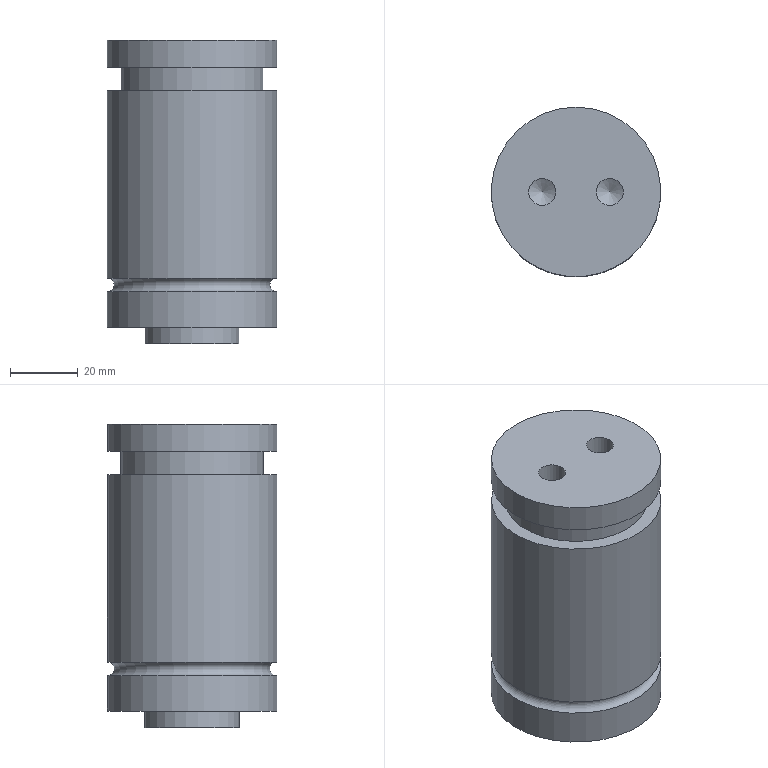Part | NX | features solid 2 | 1 solid | 15 faces | box 50.2 x 50.2 x 90 mm | volume 165612 mm3 | cylinder 7 | plane 5 | cone 2 | torus 1 | commonest cylinder face diameters 50.2 x3 8 x2 28 x1 42.2 x1
STEP:
#1=CARTESIAN_POINT('',(-615.,-166.,230.));
#2=VERTEX_POINT('',#1);
#3=CARTESIAN_POINT('',(-615.,-180.,230.));
#4=DIRECTION('',(0.,0.,1.));
#5=DIRECTION('',(0.,1.,0.));
#6=AXIS2_PLACEMENT_3D('',#3,#4,#5);
#7=CIRCLE('',#6,14.);
#8=EDGE_CURVE('',#2,#2,#7,.T.);
#9=ORIENTED_EDGE('',*,*,#8,.T.);
#10=EDGE_LOOP('',(#9));
#11=FACE_BOUND('',#10,.T.);
#12=CARTESIAN_POINT('',(-615.,-166.,235.));
#13=VERTEX_POINT('',#12);
#14=CARTESIAN_POINT('',(-615.,-180.,235.));
#15=DIRECTION('',(0.,0.,1.));
#16=DIRECTION('',(0.,1.,0.));
#17=AXIS2_PLACEMENT_3D('',#14,#15,#16);
#18=CIRCLE('',#17,14.);
#19=EDGE_CURVE('',#13,#13,#18,.T.);
#20=ORIENTED_EDGE('',*,*,#19,.F.);
#21=EDGE_LOOP('',(#20));
#22=FACE_BOUND('',#21,.T.);
#23=CARTESIAN_POINT('',(-615.,-180.,320.));
#24=DIRECTION('',(0.,0.,-1.));
#25=DIRECTION('',(0.,1.,0.));
#26=AXIS2_PLACEMENT_3D('',#23,#24,#25);
#27=CYLINDRICAL_SURFACE('',#26,14.);
#28=ADVANCED_FACE('',(#11,#22),#27,.T.);
#29=CARTESIAN_POINT('',(-615.,-154.9,235.));
#30=VERTEX_POINT('',#29);
#31=CARTESIAN_POINT('',(-615.,-180.,235.));
#32=DIRECTION('',(0.,0.,1.));
#33=DIRECTION('',(0.,1.,0.));
#34=AXIS2_PLACEMENT_3D('',#31,#32,#33);
#35=CIRCLE('',#34,25.1);
#36=EDGE_CURVE('',#30,#30,#35,.T.);
#37=ORIENTED_EDGE('',*,*,#36,.F.);
#38=EDGE_LOOP('',(#37));
#39=FACE_BOUND('',#38,.T.);
#40=ORIENTED_EDGE('',*,*,#19,.T.);
#41=EDGE_LOOP('',(#40));
#42=FACE_BOUND('',#41,.T.);
#43=CARTESIAN_POINT('',(-601.,-180.,235.));
#44=DIRECTION('',(0.,0.,-1.));
#45=DIRECTION('',(0.,1.,0.));
#46=AXIS2_PLACEMENT_3D('',#43,#44,#45);
#47=PLANE('',#46);
#48=ADVANCED_FACE('',(#39,#42),#47,.T.);
#49=ORIENTED_EDGE('',*,*,#36,.T.);
#50=EDGE_LOOP('',(#49));
#51=FACE_BOUND('',#50,.T.);
#52=CARTESIAN_POINT('',(-615.,-154.9,245.5));
#53=VERTEX_POINT('',#52);
#54=CARTESIAN_POINT('',(-615.,-180.,245.5));
#55=DIRECTION('',(0.,0.,1.));
#56=DIRECTION('',(0.,1.,0.));
#57=AXIS2_PLACEMENT_3D('',#54,#55,#56);
#58=CIRCLE('',#57,25.1);
#59=EDGE_CURVE('',#53,#53,#58,.T.);
#60=ORIENTED_EDGE('',*,*,#59,.F.);
#61=EDGE_LOOP('',(#60));
#62=FACE_BOUND('',#61,.T.);
#63=CARTESIAN_POINT('',(-615.,-180.,320.));
#64=DIRECTION('',(0.,0.,-1.));
#65=DIRECTION('',(0.,1.,0.));
#66=AXIS2_PLACEMENT_3D('',#63,#64,#65);
#67=CYLINDRICAL_SURFACE('',#66,25.1);
#68=ADVANCED_FACE('',(#51,#62),#67,.T.);
#69=ORIENTED_EDGE('',*,*,#59,.T.);
#70=EDGE_LOOP('',(#69));
#71=FACE_BOUND('',#70,.T.);
#72=CARTESIAN_POINT('',(-615.,-154.9,249.5));
#73=VERTEX_POINT('',#72);
#74=CARTESIAN_POINT('',(-615.,-180.,249.5));
#75=DIRECTION('',(0.,0.,1.));
#76=DIRECTION('',(0.,1.,0.));
#77=AXIS2_PLACEMENT_3D('',#74,#75,#76);
#78=CIRCLE('',#77,25.1);
#79=EDGE_CURVE('',#73,#73,#78,.T.);
#80=ORIENTED_EDGE('',*,*,#79,.F.);
#81=EDGE_LOOP('',(#80));
#82=FACE_BOUND('',#81,.T.);
#83=CARTESIAN_POINT('',(-615.,-180.,247.5));
#84=DIRECTION('',(0.,0.,-1.));
#85=DIRECTION('',(0.,1.,0.));
#86=AXIS2_PLACEMENT_3D('',#83,#84,#85);
#87=TOROIDAL_SURFACE('',#86,25.1,2.);
#88=ADVANCED_FACE('',(#71,#82),#87,.F.);
#89=ORIENTED_EDGE('',*,*,#79,.T.);
#90=EDGE_LOOP('',(#89));
#91=FACE_BOUND('',#90,.T.);
#92=CARTESIAN_POINT('',(-615.,-154.9,305.));
#93=VERTEX_POINT('',#92);
#94=CARTESIAN_POINT('',(-615.,-180.,305.));
#95=DIRECTION('',(0.,0.,1.));
#96=DIRECTION('',(0.,1.,0.));
#97=AXIS2_PLACEMENT_3D('',#94,#95,#96);
#98=CIRCLE('',#97,25.1);
#99=EDGE_CURVE('',#93,#93,#98,.T.);
#100=ORIENTED_EDGE('',*,*,#99,.F.);
#101=EDGE_LOOP('',(#100));
#102=FACE_BOUND('',#101,.T.);
#103=CARTESIAN_POINT('',(-615.,-180.,320.));
#104=DIRECTION('',(0.,0.,-1.));
#105=DIRECTION('',(0.,1.,0.));
#106=AXIS2_PLACEMENT_3D('',#103,#104,#105);
#107=CYLINDRICAL_SURFACE('',#106,25.1);
#108=ADVANCED_FACE('',(#91,#102),#107,.T.);
#109=ORIENTED_EDGE('',*,*,#99,.T.);
#110=EDGE_LOOP('',(#109));
#111=FACE_BOUND('',#110,.T.);
#112=CARTESIAN_POINT('',(-615.,-158.9,305.));
#113=VERTEX_POINT('',#112);
#114=CARTESIAN_POINT('',(-615.,-180.,305.));
#115=DIRECTION('',(0.,0.,1.));
#116=DIRECTION('',(0.,1.,0.));
#117=AXIS2_PLACEMENT_3D('',#114,#115,#116);
#118=CIRCLE('',#117,21.1);
#119=EDGE_CURVE('',#113,#113,#118,.T.);
#120=ORIENTED_EDGE('',*,*,#119,.F.);
#121=EDGE_LOOP('',(#120));
#122=FACE_BOUND('',#121,.T.);
#123=CARTESIAN_POINT('',(-593.9,-180.,305.));
#124=DIRECTION('',(0.,0.,-1.));
#125=DIRECTION('',(0.,1.,0.));
#126=AXIS2_PLACEMENT_3D('',#123,#124,#125);
#127=PLANE('',#126);
#128=ADVANCED_FACE('',(#111,#122),#127,.F.);
#129=ORIENTED_EDGE('',*,*,#119,.T.);
#130=EDGE_LOOP('',(#129));
#131=FACE_BOUND('',#130,.T.);
#132=CARTESIAN_POINT('',(-615.,-158.9,312.));
#133=VERTEX_POINT('',#132);
#134=CARTESIAN_POINT('',(-615.,-180.,312.));
#135=DIRECTION('',(0.,0.,1.));
#136=DIRECTION('',(0.,1.,0.));
#137=AXIS2_PLACEMENT_3D('',#134,#135,#136);
#138=CIRCLE('',#137,21.1);
#139=EDGE_CURVE('',#133,#133,#138,.T.);
#140=ORIENTED_EDGE('',*,*,#139,.F.);
#141=EDGE_LOOP('',(#140));
#142=FACE_BOUND('',#141,.T.);
#143=CARTESIAN_POINT('',(-615.,-180.,320.));
#144=DIRECTION('',(0.,0.,-1.));
#145=DIRECTION('',(0.,1.,0.));
#146=AXIS2_PLACEMENT_3D('',#143,#144,#145);
#147=CYLINDRICAL_SURFACE('',#146,21.1);
#148=ADVANCED_FACE('',(#131,#142),#147,.T.);
#149=CARTESIAN_POINT('',(-615.,-154.9,312.));
#150=VERTEX_POINT('',#149);
#151=CARTESIAN_POINT('',(-615.,-180.,312.));
#152=DIRECTION('',(0.,0.,1.));
#153=DIRECTION('',(0.,1.,0.));
#154=AXIS2_PLACEMENT_3D('',#151,#152,#153);
#155=CIRCLE('',#154,25.1);
#156=EDGE_CURVE('',#150,#150,#155,.T.);
#157=ORIENTED_EDGE('',*,*,#156,.F.);
#158=EDGE_LOOP('',(#157));
#159=FACE_BOUND('',#158,.T.);
#160=ORIENTED_EDGE('',*,*,#139,.T.);
#161=EDGE_LOOP('',(#160));
#162=FACE_BOUND('',#161,.T.);
#163=CARTESIAN_POINT('',(-593.9,-180.,312.));
#164=DIRECTION('',(0.,0.,-1.));
#165=DIRECTION('',(0.,1.,0.));
#166=AXIS2_PLACEMENT_3D('',#163,#164,#165);
#167=PLANE('',#166);
#168=ADVANCED_FACE('',(#159,#162),#167,.T.);
#169=ORIENTED_EDGE('',*,*,#156,.T.);
#170=EDGE_LOOP('',(#169));
#171=FACE_BOUND('',#170,.T.);
#172=CARTESIAN_POINT('',(-615.,-154.9,320.));
#173=VERTEX_POINT('',#172);
#174=CARTESIAN_POINT('',(-615.,-180.,320.));
#175=DIRECTION('',(0.,0.,1.));
#176=DIRECTION('',(0.,1.,0.));
#177=AXIS2_PLACEMENT_3D('',#174,#175,#176);
#178=CIRCLE('',#177,25.1);
#179=EDGE_CURVE('',#173,#173,#178,.T.);
#180=ORIENTED_EDGE('',*,*,#179,.F.);
#181=EDGE_LOOP('',(#180));
#182=FACE_BOUND('',#181,.T.);
#183=CARTESIAN_POINT('',(-615.,-180.,320.));
#184=DIRECTION('',(0.,0.,-1.));
#185=DIRECTION('',(0.,1.,0.));
#186=AXIS2_PLACEMENT_3D('',#183,#184,#185);
#187=CYLINDRICAL_SURFACE('',#186,25.1);
#188=ADVANCED_FACE('',(#171,#182),#187,.T.);
#189=CARTESIAN_POINT('',(-601.,-180.,320.));
#190=VERTEX_POINT('',#189);
#191=CARTESIAN_POINT('',(-605.,-180.,320.));
#192=DIRECTION('',(0.,0.,1.));
#193=DIRECTION('',(1.,0.,0.));
#194=AXIS2_PLACEMENT_3D('',#191,#192,#193);
#195=CIRCLE('',#194,4.);
#196=EDGE_CURVE('',#190,#190,#195,.T.);
#197=ORIENTED_EDGE('',*,*,#196,.F.);
#198=EDGE_LOOP('',(#197));
#199=FACE_BOUND('',#198,.T.);
#200=CARTESIAN_POINT('',(-621.,-180.,320.));
#201=VERTEX_POINT('',#200);
#202=CARTESIAN_POINT('',(-625.,-180.,320.));
#203=DIRECTION('',(0.,0.,1.));
#204=DIRECTION('',(1.,0.,0.));
#205=AXIS2_PLACEMENT_3D('',#202,#203,#204);
#206=CIRCLE('',#205,4.);
#207=EDGE_CURVE('',#201,#201,#206,.T.);
#208=ORIENTED_EDGE('',*,*,#207,.F.);
#209=EDGE_LOOP('',(#208));
#210=FACE_BOUND('',#209,.T.);
#211=ORIENTED_EDGE('',*,*,#179,.T.);
#212=EDGE_LOOP('',(#211));
#213=FACE_BOUND('',#212,.T.);
#214=CARTESIAN_POINT('',(-615.,-180.,320.));
#215=DIRECTION('',(0.,0.,-1.));
#216=DIRECTION('',(0.,1.,0.));
#217=AXIS2_PLACEMENT_3D('',#214,#215,#216);
#218=PLANE('',#217);
#219=ADVANCED_FACE('',(#199,#210,#213),#218,.F.);
#220=ORIENTED_EDGE('',*,*,#8,.F.);
#221=EDGE_LOOP('',(#220));
#222=FACE_BOUND('',#221,.T.);
#223=CARTESIAN_POINT('',(-615.,-180.,230.));
#224=DIRECTION('',(0.,0.,-1.));
#225=DIRECTION('',(0.,1.,0.));
#226=AXIS2_PLACEMENT_3D('',#223,#224,#225);
#227=PLANE('',#226);
#228=ADVANCED_FACE('',(#222),#227,.T.);
#229=CARTESIAN_POINT('',(-621.,-180.,314.));
#230=VERTEX_POINT('',#229);
#231=CARTESIAN_POINT('',(-625.,-180.,314.));
#232=DIRECTION('',(0.,0.,1.));
#233=DIRECTION('',(1.,0.,0.));
#234=AXIS2_PLACEMENT_3D('',#231,#232,#233);
#235=CIRCLE('',#234,4.);
#236=EDGE_CURVE('',#230,#230,#235,.T.);
#237=ORIENTED_EDGE('',*,*,#236,.T.);
#238=EDGE_LOOP('',(#237));
#239=FACE_BOUND('',#238,.T.);
#240=CARTESIAN_POINT('',(-625.,-180.,311.691));
#241=VERTEX_POINT('',#240);
#242=VERTEX_LOOP('',#241);
#243=FACE_BOUND('',#242,.T.);
#244=CARTESIAN_POINT('',(-625.,-180.,314.));
#245=DIRECTION('',(0.,0.,1.));
#246=DIRECTION('',(-1.,0.,0.));
#247=AXIS2_PLACEMENT_3D('',#244,#245,#246);
#248=CONICAL_SURFACE('',#247,4.,1.047);
#249=ADVANCED_FACE('',(#239,#243),#248,.F.);
#250=ORIENTED_EDGE('',*,*,#236,.F.);
#251=EDGE_LOOP('',(#250));
#252=FACE_BOUND('',#251,.T.);
#253=ORIENTED_EDGE('',*,*,#207,.T.);
#254=EDGE_LOOP('',(#253));
#255=FACE_BOUND('',#254,.T.);
#256=CARTESIAN_POINT('',(-625.,-180.,320.));
#257=DIRECTION('',(0.,0.,-1.));
#258=DIRECTION('',(1.,0.,0.));
#259=AXIS2_PLACEMENT_3D('',#256,#257,#258);
#260=CYLINDRICAL_SURFACE('',#259,4.);
#261=ADVANCED_FACE('',(#252,#255),#260,.F.);
#262=CARTESIAN_POINT('',(-601.,-180.,314.));
#263=VERTEX_POINT('',#262);
#264=CARTESIAN_POINT('',(-605.,-180.,314.));
#265=DIRECTION('',(0.,0.,1.));
#266=DIRECTION('',(1.,0.,0.));
#267=AXIS2_PLACEMENT_3D('',#264,#265,#266);
#268=CIRCLE('',#267,4.);
#269=EDGE_CURVE('',#263,#263,#268,.T.);
#270=ORIENTED_EDGE('',*,*,#269,.T.);
#271=EDGE_LOOP('',(#270));
#272=FACE_BOUND('',#271,.T.);
#273=CARTESIAN_POINT('',(-605.,-180.,311.691));
#274=VERTEX_POINT('',#273);
#275=VERTEX_LOOP('',#274);
#276=FACE_BOUND('',#275,.T.);
#277=CARTESIAN_POINT('',(-605.,-180.,314.));
#278=DIRECTION('',(0.,0.,1.));
#279=DIRECTION('',(-1.,0.,0.));
#280=AXIS2_PLACEMENT_3D('',#277,#278,#279);
#281=CONICAL_SURFACE('',#280,4.,1.047);
#282=ADVANCED_FACE('',(#272,#276),#281,.F.);
#283=ORIENTED_EDGE('',*,*,#269,.F.);
#284=EDGE_LOOP('',(#283));
#285=FACE_BOUND('',#284,.T.);
#286=ORIENTED_EDGE('',*,*,#196,.T.);
#287=EDGE_LOOP('',(#286));
#288=FACE_BOUND('',#287,.T.);
#289=CARTESIAN_POINT('',(-605.,-180.,320.));
#290=DIRECTION('',(0.,0.,-1.));
#291=DIRECTION('',(1.,0.,0.));
#292=AXIS2_PLACEMENT_3D('',#289,#290,#291);
#293=CYLINDRICAL_SURFACE('',#292,4.);
#294=ADVANCED_FACE('',(#285,#288),#293,.F.);
#295=CLOSED_SHELL('',(#28,#48,#68,#88,#108,#128,#148,#168,#188,#219,#228,#249,#261,#282,#294));
#296=MANIFOLD_SOLID_BREP('',#295);
#297=(LENGTH_UNIT()NAMED_UNIT(*)SI_UNIT(.MILLI.,.METRE.));
#298=UNCERTAINTY_MEASURE_WITH_UNIT(LENGTH_MEASURE(0.00001),#297,'','');
#299=(NAMED_UNIT(*)PLANE_ANGLE_UNIT()SI_UNIT($,.RADIAN.));
#300=(NAMED_UNIT(*)SI_UNIT($,.STERADIAN.)SOLID_ANGLE_UNIT());
#301=(GEOMETRIC_REPRESENTATION_CONTEXT(3)GLOBAL_UNCERTAINTY_ASSIGNED_CONTEXT((#298))GLOBAL_UNIT_ASSIGNED_CONTEXT((#297,#299,#300))REPRESENTATION_CONTEXT('',''));
#302=ADVANCED_BREP_SHAPE_REPRESENTATION('',(#296),#301);